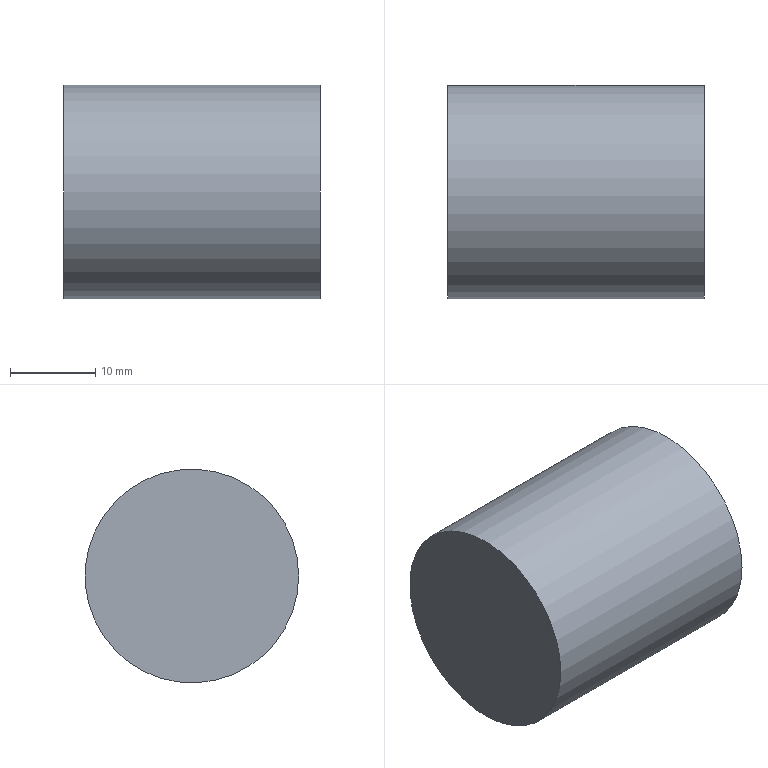Part | NX | features solid 2 | 1 solid | 5 faces | box 30 x 25 x 25 mm | volume 7799 mm3 | plane 3 | cylinder 2 | commonest cylinder face diameters 21 x1 25 x1
STEP:
#1=CARTESIAN_POINT('',(1122.,-168.5,-405.));
#2=VERTEX_POINT('',#1);
#3=CARTESIAN_POINT('',(1122.,-156.,-405.));
#4=DIRECTION('',(1.,0.,0.));
#5=DIRECTION('',(0.,-1.,0.));
#6=AXIS2_PLACEMENT_3D('',#3,#4,#5);
#7=CIRCLE('',#6,12.5);
#8=EDGE_CURVE('',#2,#2,#7,.T.);
#9=ORIENTED_EDGE('',*,*,#8,.F.);
#10=EDGE_LOOP('',(#9));
#11=FACE_BOUND('',#10,.T.);
#12=CARTESIAN_POINT('',(1092.,-168.5,-405.));
#13=VERTEX_POINT('',#12);
#14=CARTESIAN_POINT('',(1092.,-156.,-405.));
#15=DIRECTION('',(1.,0.,0.));
#16=DIRECTION('',(0.,-1.,0.));
#17=AXIS2_PLACEMENT_3D('',#14,#15,#16);
#18=CIRCLE('',#17,12.5);
#19=EDGE_CURVE('',#13,#13,#18,.T.);
#20=ORIENTED_EDGE('',*,*,#19,.T.);
#21=EDGE_LOOP('',(#20));
#22=FACE_BOUND('',#21,.T.);
#23=CARTESIAN_POINT('',(1132.,-156.,-405.));
#24=DIRECTION('',(-1.,0.,0.));
#25=DIRECTION('',(0.,1.,0.));
#26=AXIS2_PLACEMENT_3D('',#23,#24,#25);
#27=CYLINDRICAL_SURFACE('',#26,12.5);
#28=ADVANCED_FACE('',(#11,#22),#27,.T.);
#29=CARTESIAN_POINT('',(1122.,-166.5,-405.));
#30=VERTEX_POINT('',#29);
#31=CARTESIAN_POINT('',(1122.,-156.,-405.));
#32=DIRECTION('',(1.,0.,0.));
#33=DIRECTION('',(0.,-1.,0.));
#34=AXIS2_PLACEMENT_3D('',#31,#32,#33);
#35=CIRCLE('',#34,10.5);
#36=EDGE_CURVE('',#30,#30,#35,.T.);
#37=ORIENTED_EDGE('',*,*,#36,.F.);
#38=EDGE_LOOP('',(#37));
#39=FACE_BOUND('',#38,.T.);
#40=ORIENTED_EDGE('',*,*,#8,.T.);
#41=EDGE_LOOP('',(#40));
#42=FACE_BOUND('',#41,.T.);
#43=CARTESIAN_POINT('',(1122.,-156.,-405.));
#44=DIRECTION('',(1.,0.,0.));
#45=DIRECTION('',(0.,-1.,0.));
#46=AXIS2_PLACEMENT_3D('',#43,#44,#45);
#47=PLANE('',#46);
#48=ADVANCED_FACE('',(#39,#42),#47,.T.);
#49=ORIENTED_EDGE('',*,*,#19,.F.);
#50=EDGE_LOOP('',(#49));
#51=FACE_BOUND('',#50,.T.);
#52=CARTESIAN_POINT('',(1092.,-156.,-405.));
#53=DIRECTION('',(1.,0.,0.));
#54=DIRECTION('',(0.,-1.,0.));
#55=AXIS2_PLACEMENT_3D('',#52,#53,#54);
#56=PLANE('',#55);
#57=ADVANCED_FACE('',(#51),#56,.F.);
#58=ORIENTED_EDGE('',*,*,#36,.T.);
#59=EDGE_LOOP('',(#58));
#60=FACE_BOUND('',#59,.T.);
#61=CARTESIAN_POINT('',(1102.,-166.5,-405.));
#62=VERTEX_POINT('',#61);
#63=CARTESIAN_POINT('',(1102.,-156.,-405.));
#64=DIRECTION('',(1.,0.,0.));
#65=DIRECTION('',(0.,-1.,0.));
#66=AXIS2_PLACEMENT_3D('',#63,#64,#65);
#67=CIRCLE('',#66,10.5);
#68=EDGE_CURVE('',#62,#62,#67,.T.);
#69=ORIENTED_EDGE('',*,*,#68,.F.);
#70=EDGE_LOOP('',(#69));
#71=FACE_BOUND('',#70,.T.);
#72=CARTESIAN_POINT('',(1102.,-156.,-405.));
#73=DIRECTION('',(1.,0.,0.));
#74=DIRECTION('',(0.,-1.,0.));
#75=AXIS2_PLACEMENT_3D('',#72,#73,#74);
#76=CYLINDRICAL_SURFACE('',#75,10.5);
#77=ADVANCED_FACE('',(#60,#71),#76,.F.);
#78=ORIENTED_EDGE('',*,*,#68,.T.);
#79=EDGE_LOOP('',(#78));
#80=FACE_BOUND('',#79,.T.);
#81=CARTESIAN_POINT('',(1102.,-156.,-405.));
#82=DIRECTION('',(1.,0.,0.));
#83=DIRECTION('',(0.,-1.,0.));
#84=AXIS2_PLACEMENT_3D('',#81,#82,#83);
#85=PLANE('',#84);
#86=ADVANCED_FACE('',(#80),#85,.T.);
#87=CLOSED_SHELL('',(#28,#48,#57,#77,#86));
#88=MANIFOLD_SOLID_BREP('',#87);
#89=(LENGTH_UNIT()NAMED_UNIT(*)SI_UNIT(.MILLI.,.METRE.));
#90=UNCERTAINTY_MEASURE_WITH_UNIT(LENGTH_MEASURE(0.00001),#89,'','');
#91=(NAMED_UNIT(*)PLANE_ANGLE_UNIT()SI_UNIT($,.RADIAN.));
#92=(NAMED_UNIT(*)SI_UNIT($,.STERADIAN.)SOLID_ANGLE_UNIT());
#93=(GEOMETRIC_REPRESENTATION_CONTEXT(3)GLOBAL_UNCERTAINTY_ASSIGNED_CONTEXT((#90))GLOBAL_UNIT_ASSIGNED_CONTEXT((#89,#91,#92))REPRESENTATION_CONTEXT('',''));
#94=ADVANCED_BREP_SHAPE_REPRESENTATION('',(#88),#93);